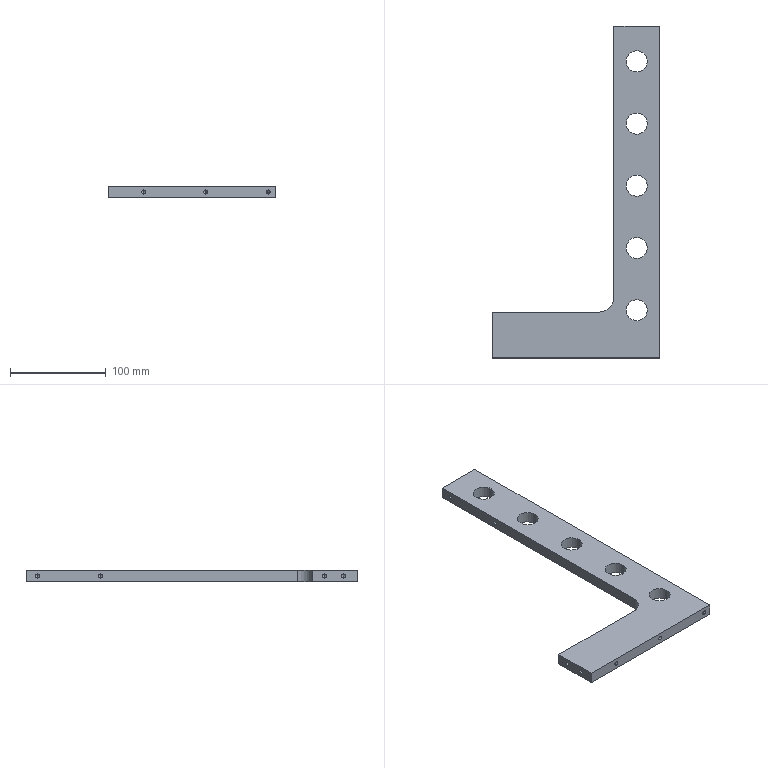Part | STEP file | 2043 Reinforcing rib 2 | 1 solid | 63 faces | box 175 x 347 x 12 mm | volume 248598 mm3 | cylinder 33 | cone 22 | plane 8 | commonest cylinder face diameters 4.2 x22 22 x10 30 x1